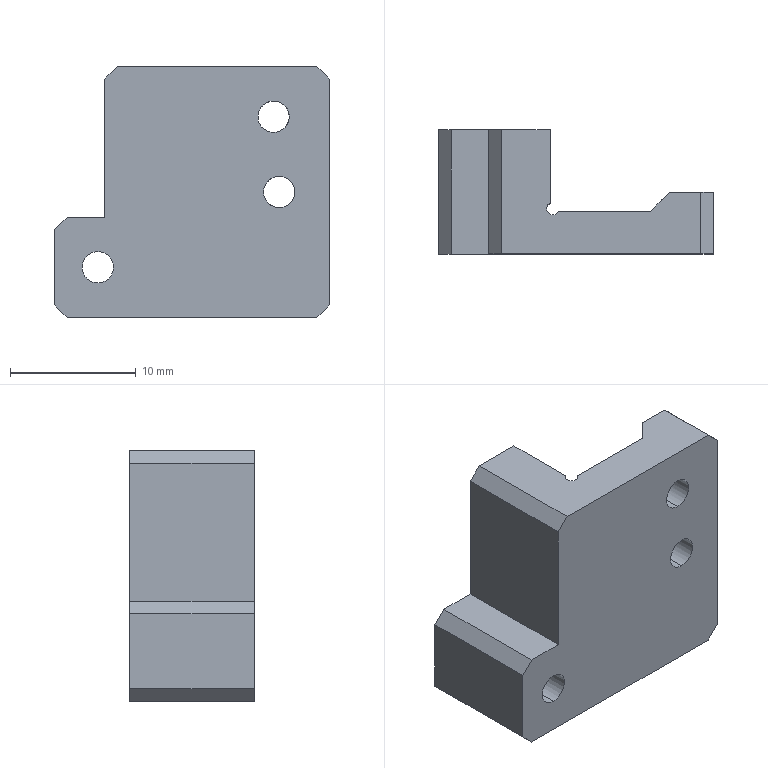Part | SolidWorks | features HoleWzd 3, ICE 2, MoveFace 2, Chamfer 1, Extrusion 1 | 1 solid | 31 faces | box 21.9 x 9.9 x 20 mm | volume 2171 mm3 | plane 19 | cylinder 10 | cone 2 | commonest cylinder face diameters 2.5 x6 1 x2 1.5 x2
STEP:
#1=CARTESIAN_POINT('',(11.9,1.75,5.75));
#2=VERTEX_POINT('',#1);
#3=CARTESIAN_POINT('',(11.9,1.75,4.25));
#4=VERTEX_POINT('',#3);
#5=CARTESIAN_POINT('',(11.9,1.75,5.));
#6=DIRECTION('',(1.,0.,0.));
#7=DIRECTION('',(0.,0.,-1.));
#8=AXIS2_PLACEMENT_3D('',#5,#6,#7);
#9=CIRCLE('',#8,0.75);
#10=EDGE_CURVE('',#2,#4,#9,.T.);
#11=ORIENTED_EDGE('',*,*,#10,.F.);
#12=CARTESIAN_POINT('',(17.9,1.75,5.75));
#13=VERTEX_POINT('',#12);
#14=CARTESIAN_POINT('',(17.9,1.75,5.75));
#15=DIRECTION('',(1.,0.,0.));
#16=VECTOR('',#15,1000.);
#17=LINE('',#14,#16);
#18=EDGE_CURVE('',#2,#13,#17,.T.);
#19=ORIENTED_EDGE('',*,*,#18,.T.);
#20=CARTESIAN_POINT('',(17.9,1.75,4.25));
#21=VERTEX_POINT('',#20);
#22=CARTESIAN_POINT('',(17.9,1.75,5.));
#23=DIRECTION('',(1.,0.,0.));
#24=DIRECTION('',(0.,0.,-1.));
#25=AXIS2_PLACEMENT_3D('',#22,#23,#24);
#26=CIRCLE('',#25,0.75);
#27=EDGE_CURVE('',#13,#21,#26,.T.);
#28=ORIENTED_EDGE('',*,*,#27,.T.);
#29=CARTESIAN_POINT('',(17.9,1.75,4.25));
#30=DIRECTION('',(1.,0.,0.));
#31=VECTOR('',#30,1000.);
#32=LINE('',#29,#31);
#33=EDGE_CURVE('',#4,#21,#32,.T.);
#34=ORIENTED_EDGE('',*,*,#33,.F.);
#35=EDGE_LOOP('',(#11,#19,#28,#34));
#36=FACE_OUTER_BOUND('',#35,.T.);
#37=CARTESIAN_POINT('',(17.9,1.75,5.));
#38=DIRECTION('',(1.,0.,0.));
#39=DIRECTION('',(0.,0.,-1.));
#40=AXIS2_PLACEMENT_3D('',#37,#38,#39);
#41=CYLINDRICAL_SURFACE('',#40,0.75);
#42=ADVANCED_FACE('',(#36),#41,.F.);
#43=CARTESIAN_POINT('',(11.449,1.75,5.));
#44=VERTEX_POINT('',#43);
#45=CARTESIAN_POINT('',(11.9,1.75,4.25));
#46=DIRECTION('',(0.515,0.,-0.8572));
#47=VECTOR('',#46,1000.);
#48=LINE('',#45,#47);
#49=EDGE_CURVE('',#44,#4,#48,.T.);
#50=ORIENTED_EDGE('',*,*,#49,.F.);
#51=CARTESIAN_POINT('',(11.9,1.75,5.75));
#52=DIRECTION('',(0.515,0.,0.8572));
#53=VECTOR('',#52,1000.);
#54=LINE('',#51,#53);
#55=EDGE_CURVE('',#44,#2,#54,.T.);
#56=ORIENTED_EDGE('',*,*,#55,.T.);
#57=ORIENTED_EDGE('',*,*,#10,.T.);
#58=EDGE_LOOP('',(#50,#56,#57));
#59=FACE_OUTER_BOUND('',#58,.T.);
#60=CARTESIAN_POINT('',(11.9,1.75,5.));
#61=DIRECTION('',(1.,0.,0.));
#62=DIRECTION('',(0.,0.,-1.));
#63=AXIS2_PLACEMENT_3D('',#60,#61,#62);
#64=CONICAL_SURFACE('',#63,0.75,1.03);
#65=ADVANCED_FACE('',(#59),#64,.F.);
#66=CARTESIAN_POINT('',(12.9,3.4,17.122));
#67=VERTEX_POINT('',#66);
#68=CARTESIAN_POINT('',(13.45,3.95,17.25));
#69=VERTEX_POINT('',#68);
#70=CARTESIAN_POINT('',(12.9,3.4,17.122));
#71=CARTESIAN_POINT('',(13.072,3.572,17.207));
#72=CARTESIAN_POINT('',(13.259,3.759,17.25));
#73=CARTESIAN_POINT('',(13.45,3.95,17.25));
#74=(BOUNDED_CURVE()B_SPLINE_CURVE(3,(#70,#71,#72,#73),.UNSPECIFIED.,.F.,.F.)B_SPLINE_CURVE_WITH_KNOTS((4,4),(1.115,1.571),.UNSPECIFIED.)CURVE()GEOMETRIC_REPRESENTATION_ITEM()RATIONAL_B_SPLINE_CURVE((1.,0.9828,0.9828,1.))REPRESENTATION_ITEM(''));
#75=EDGE_CURVE('',#67,#69,#74,.T.);
#76=ORIENTED_EDGE('',*,*,#75,.T.);
#77=CARTESIAN_POINT('',(13.45,0.,17.25));
#78=VERTEX_POINT('',#77);
#79=CARTESIAN_POINT('',(13.45,0.,17.25));
#80=DIRECTION('',(0.,-1.,0.));
#81=VECTOR('',#80,1000.);
#82=LINE('',#79,#81);
#83=EDGE_CURVE('',#69,#78,#82,.T.);
#84=ORIENTED_EDGE('',*,*,#83,.T.);
#85=CARTESIAN_POINT('',(13.45,0.,14.75));
#86=VERTEX_POINT('',#85);
#87=CARTESIAN_POINT('',(13.45,0.,16.));
#88=DIRECTION('',(0.,-1.,0.));
#89=DIRECTION('',(0.,0.,-1.));
#90=AXIS2_PLACEMENT_3D('',#87,#88,#89);
#91=CIRCLE('',#90,1.25);
#92=EDGE_CURVE('',#78,#86,#91,.T.);
#93=ORIENTED_EDGE('',*,*,#92,.T.);
#94=CARTESIAN_POINT('',(13.45,3.95,14.75));
#95=VERTEX_POINT('',#94);
#96=CARTESIAN_POINT('',(13.45,0.,14.75));
#97=DIRECTION('',(0.,-1.,0.));
#98=VECTOR('',#97,1000.);
#99=LINE('',#96,#98);
#100=EDGE_CURVE('',#95,#86,#99,.T.);
#101=ORIENTED_EDGE('',*,*,#100,.F.);
#102=CARTESIAN_POINT('',(12.9,3.4,14.878));
#103=VERTEX_POINT('',#102);
#104=CARTESIAN_POINT('',(13.45,3.95,14.75));
#105=CARTESIAN_POINT('',(13.259,3.759,14.75));
#106=CARTESIAN_POINT('',(13.072,3.572,14.793));
#107=CARTESIAN_POINT('',(12.9,3.4,14.878));
#108=(BOUNDED_CURVE()B_SPLINE_CURVE(3,(#104,#105,#106,#107),.UNSPECIFIED.,.F.,.F.)B_SPLINE_CURVE_WITH_KNOTS((4,4),(4.712,5.168),.UNSPECIFIED.)CURVE()GEOMETRIC_REPRESENTATION_ITEM()RATIONAL_B_SPLINE_CURVE((1.,0.9828,0.9828,1.))REPRESENTATION_ITEM(''));
#109=EDGE_CURVE('',#95,#103,#108,.T.);
#110=ORIENTED_EDGE('',*,*,#109,.T.);
#111=CARTESIAN_POINT('',(13.45,3.4,16.));
#112=DIRECTION('',(0.,-1.,0.));
#113=DIRECTION('',(1.,0.,0.));
#114=AXIS2_PLACEMENT_3D('',#111,#112,#113);
#115=CIRCLE('',#114,1.25);
#116=EDGE_CURVE('',#67,#103,#115,.T.);
#117=ORIENTED_EDGE('',*,*,#116,.F.);
#118=EDGE_LOOP('',(#76,#84,#93,#101,#110,#117));
#119=FACE_OUTER_BOUND('',#118,.T.);
#120=CARTESIAN_POINT('',(13.45,0.,16.));
#121=DIRECTION('',(0.,-1.,0.));
#122=DIRECTION('',(0.,0.,-1.));
#123=AXIS2_PLACEMENT_3D('',#120,#121,#122);
#124=CYLINDRICAL_SURFACE('',#123,1.25);
#125=ADVANCED_FACE('',(#119),#124,.F.);
#126=CARTESIAN_POINT('',(-0.55,9.9,5.25));
#127=VERTEX_POINT('',#126);
#128=CARTESIAN_POINT('',(-0.55,9.9,2.75));
#129=VERTEX_POINT('',#128);
#130=CARTESIAN_POINT('',(-0.55,9.9,4.));
#131=DIRECTION('',(0.,-1.,0.));
#132=DIRECTION('',(0.,0.,-1.));
#133=AXIS2_PLACEMENT_3D('',#130,#131,#132);
#134=CIRCLE('',#133,1.25);
#135=EDGE_CURVE('',#127,#129,#134,.T.);
#136=ORIENTED_EDGE('',*,*,#135,.F.);
#137=CARTESIAN_POINT('',(-0.55,0.,5.25));
#138=VERTEX_POINT('',#137);
#139=CARTESIAN_POINT('',(-0.55,0.,5.25));
#140=DIRECTION('',(0.,-1.,0.));
#141=VECTOR('',#140,1000.);
#142=LINE('',#139,#141);
#143=EDGE_CURVE('',#127,#138,#142,.T.);
#144=ORIENTED_EDGE('',*,*,#143,.T.);
#145=CARTESIAN_POINT('',(-0.55,0.,2.75));
#146=VERTEX_POINT('',#145);
#147=CARTESIAN_POINT('',(-0.55,0.,4.));
#148=DIRECTION('',(0.,-1.,0.));
#149=DIRECTION('',(0.,0.,-1.));
#150=AXIS2_PLACEMENT_3D('',#147,#148,#149);
#151=CIRCLE('',#150,1.25);
#152=EDGE_CURVE('',#138,#146,#151,.T.);
#153=ORIENTED_EDGE('',*,*,#152,.T.);
#154=CARTESIAN_POINT('',(-0.55,0.,2.75));
#155=DIRECTION('',(0.,-1.,0.));
#156=VECTOR('',#155,1000.);
#157=LINE('',#154,#156);
#158=EDGE_CURVE('',#129,#146,#157,.T.);
#159=ORIENTED_EDGE('',*,*,#158,.F.);
#160=EDGE_LOOP('',(#136,#144,#153,#159));
#161=FACE_OUTER_BOUND('',#160,.T.);
#162=CARTESIAN_POINT('',(-0.55,0.,4.));
#163=DIRECTION('',(0.,-1.,0.));
#164=DIRECTION('',(0.,0.,-1.));
#165=AXIS2_PLACEMENT_3D('',#162,#163,#164);
#166=CYLINDRICAL_SURFACE('',#165,1.25);
#167=ADVANCED_FACE('',(#161),#166,.F.);
#168=CARTESIAN_POINT('',(12.9,3.4,10.75));
#169=VERTEX_POINT('',#168);
#170=CARTESIAN_POINT('',(13.9,4.4,11.25));
#171=VERTEX_POINT('',#170);
#172=CARTESIAN_POINT('',(12.9,3.4,10.75));
#173=CARTESIAN_POINT('',(13.141,3.641,11.071));
#174=CARTESIAN_POINT('',(13.499,3.999,11.25));
#175=CARTESIAN_POINT('',(13.9,4.4,11.25));
#176=(BOUNDED_CURVE()B_SPLINE_CURVE(3,(#172,#173,#174,#175),.UNSPECIFIED.,.F.,.F.)B_SPLINE_CURVE_WITH_KNOTS((4,4),(0.6435,1.571),.UNSPECIFIED.)CURVE()GEOMETRIC_REPRESENTATION_ITEM()RATIONAL_B_SPLINE_CURVE((1.,0.9296,0.9296,1.))REPRESENTATION_ITEM(''));
#177=EDGE_CURVE('',#169,#171,#176,.T.);
#178=ORIENTED_EDGE('',*,*,#177,.T.);
#179=CARTESIAN_POINT('',(13.9,0.,11.25));
#180=VERTEX_POINT('',#179);
#181=CARTESIAN_POINT('',(13.9,0.,11.25));
#182=DIRECTION('',(0.,-1.,0.));
#183=VECTOR('',#182,1000.);
#184=LINE('',#181,#183);
#185=EDGE_CURVE('',#171,#180,#184,.T.);
#186=ORIENTED_EDGE('',*,*,#185,.T.);
#187=CARTESIAN_POINT('',(13.9,0.,8.75));
#188=VERTEX_POINT('',#187);
#189=CARTESIAN_POINT('',(13.9,0.,10.));
#190=DIRECTION('',(0.,-1.,0.));
#191=DIRECTION('',(0.,0.,-1.));
#192=AXIS2_PLACEMENT_3D('',#189,#190,#191);
#193=CIRCLE('',#192,1.25);
#194=EDGE_CURVE('',#180,#188,#193,.T.);
#195=ORIENTED_EDGE('',*,*,#194,.T.);
#196=CARTESIAN_POINT('',(13.9,4.4,8.75));
#197=VERTEX_POINT('',#196);
#198=CARTESIAN_POINT('',(13.9,0.,8.75));
#199=DIRECTION('',(0.,-1.,0.));
#200=VECTOR('',#199,1000.);
#201=LINE('',#198,#200);
#202=EDGE_CURVE('',#197,#188,#201,.T.);
#203=ORIENTED_EDGE('',*,*,#202,.F.);
#204=CARTESIAN_POINT('',(12.9,3.4,9.25));
#205=VERTEX_POINT('',#204);
#206=CARTESIAN_POINT('',(13.9,4.4,8.75));
#207=CARTESIAN_POINT('',(13.499,3.999,8.75));
#208=CARTESIAN_POINT('',(13.141,3.641,8.929));
#209=CARTESIAN_POINT('',(12.9,3.4,9.25));
#210=(BOUNDED_CURVE()B_SPLINE_CURVE(3,(#206,#207,#208,#209),.UNSPECIFIED.,.F.,.T.)B_SPLINE_CURVE_WITH_KNOTS((4,4),(4.712,5.64),.UNSPECIFIED.)CURVE()GEOMETRIC_REPRESENTATION_ITEM()RATIONAL_B_SPLINE_CURVE((1.,0.9296,0.9296,1.))REPRESENTATION_ITEM(''));
#211=EDGE_CURVE('',#197,#205,#210,.T.);
#212=ORIENTED_EDGE('',*,*,#211,.T.);
#213=CARTESIAN_POINT('',(13.9,3.4,10.));
#214=DIRECTION('',(0.,-1.,0.));
#215=DIRECTION('',(1.,0.,0.));
#216=AXIS2_PLACEMENT_3D('',#213,#214,#215);
#217=CIRCLE('',#216,1.25);
#218=EDGE_CURVE('',#169,#205,#217,.T.);
#219=ORIENTED_EDGE('',*,*,#218,.F.);
#220=EDGE_LOOP('',(#178,#186,#195,#203,#212,#219));
#221=FACE_OUTER_BOUND('',#220,.T.);
#222=CARTESIAN_POINT('',(13.9,0.,10.));
#223=DIRECTION('',(0.,-1.,0.));
#224=DIRECTION('',(0.,0.,-1.));
#225=AXIS2_PLACEMENT_3D('',#222,#223,#224);
#226=CYLINDRICAL_SURFACE('',#225,1.25);
#227=ADVANCED_FACE('',(#221),#226,.F.);
#228=CARTESIAN_POINT('',(4.6,3.6,20.));
#229=VERTEX_POINT('',#228);
#230=CARTESIAN_POINT('',(4.9,4.058,20.));
#231=VERTEX_POINT('',#230);
#232=CARTESIAN_POINT('',(5.1,3.6,20.));
#233=DIRECTION('',(0.,0.,-1.));
#234=DIRECTION('',(1.,0.,0.));
#235=AXIS2_PLACEMENT_3D('',#232,#233,#234);
#236=CIRCLE('',#235,0.5);
#237=EDGE_CURVE('',#229,#231,#236,.T.);
#238=ORIENTED_EDGE('',*,*,#237,.F.);
#239=CARTESIAN_POINT('',(4.6,3.6,0.));
#240=VERTEX_POINT('',#239);
#241=CARTESIAN_POINT('',(4.6,3.6,20.));
#242=DIRECTION('',(0.,0.,-1.));
#243=VECTOR('',#242,1000.);
#244=LINE('',#241,#243);
#245=EDGE_CURVE('',#229,#240,#244,.T.);
#246=ORIENTED_EDGE('',*,*,#245,.T.);
#247=CARTESIAN_POINT('',(4.9,4.058,0.));
#248=VERTEX_POINT('',#247);
#249=CARTESIAN_POINT('',(5.1,3.6,0.));
#250=DIRECTION('',(0.,0.,-1.));
#251=DIRECTION('',(1.,0.,0.));
#252=AXIS2_PLACEMENT_3D('',#249,#250,#251);
#253=CIRCLE('',#252,0.5);
#254=EDGE_CURVE('',#240,#248,#253,.T.);
#255=ORIENTED_EDGE('',*,*,#254,.T.);
#256=CARTESIAN_POINT('',(4.9,4.058,20.));
#257=DIRECTION('',(0.,0.,-1.));
#258=VECTOR('',#257,1000.);
#259=LINE('',#256,#258);
#260=EDGE_CURVE('',#231,#248,#259,.T.);
#261=ORIENTED_EDGE('',*,*,#260,.F.);
#262=EDGE_LOOP('',(#238,#246,#255,#261));
#263=FACE_OUTER_BOUND('',#262,.T.);
#264=CARTESIAN_POINT('',(5.1,3.6,20.));
#265=DIRECTION('',(0.,0.,-1.));
#266=DIRECTION('',(-1.,0.,0.));
#267=AXIS2_PLACEMENT_3D('',#264,#265,#266);
#268=CYLINDRICAL_SURFACE('',#267,0.5);
#269=ADVANCED_FACE('',(#263),#268,.F.);
#270=ORIENTED_EDGE('',*,*,#75,.F.);
#271=CARTESIAN_POINT('',(12.9,3.4,20.));
#272=VERTEX_POINT('',#271);
#273=CARTESIAN_POINT('',(12.9,3.4,25.22));
#274=DIRECTION('',(0.,0.,-1.));
#275=VECTOR('',#274,1000.);
#276=LINE('',#273,#275);
#277=EDGE_CURVE('',#272,#67,#276,.T.);
#278=ORIENTED_EDGE('',*,*,#277,.F.);
#279=CARTESIAN_POINT('',(14.4,4.9,20.));
#280=VERTEX_POINT('',#279);
#281=CARTESIAN_POINT('',(14.4,4.9,20.));
#282=DIRECTION('',(0.7071,0.7071,0.));
#283=VECTOR('',#282,1000.);
#284=LINE('',#281,#283);
#285=EDGE_CURVE('',#272,#280,#284,.T.);
#286=ORIENTED_EDGE('',*,*,#285,.T.);
#287=CARTESIAN_POINT('',(14.4,4.9,16.812));
#288=VERTEX_POINT('',#287);
#289=CARTESIAN_POINT('',(14.4,4.9,25.22));
#290=DIRECTION('',(0.,0.,-1.));
#291=VECTOR('',#290,1000.);
#292=LINE('',#289,#291);
#293=EDGE_CURVE('',#280,#288,#292,.T.);
#294=ORIENTED_EDGE('',*,*,#293,.T.);
#295=CARTESIAN_POINT('',(13.45,3.95,17.25));
#296=CARTESIAN_POINT('',(13.821,4.321,17.25));
#297=CARTESIAN_POINT('',(14.159,4.659,17.095));
#298=CARTESIAN_POINT('',(14.4,4.9,16.812));
#299=(BOUNDED_CURVE()B_SPLINE_CURVE(3,(#295,#296,#297,#298),.UNSPECIFIED.,.F.,.T.)B_SPLINE_CURVE_WITH_KNOTS((4,4),(1.571,2.434),.UNSPECIFIED.)CURVE()GEOMETRIC_REPRESENTATION_ITEM()RATIONAL_B_SPLINE_CURVE((1.,0.9388,0.9388,1.))REPRESENTATION_ITEM(''));
#300=EDGE_CURVE('',#69,#288,#299,.T.);
#301=ORIENTED_EDGE('',*,*,#300,.F.);
#302=EDGE_LOOP('',(#270,#278,#286,#294,#301));
#303=FACE_OUTER_BOUND('',#302,.T.);
#304=CARTESIAN_POINT('',(14.4,4.9,25.22));
#305=DIRECTION('',(-0.7071,0.7071,0.));
#306=DIRECTION('',(-0.7071,-0.7071,0.));
#307=AXIS2_PLACEMENT_3D('',#304,#305,#306);
#308=PLANE('',#307);
#309=ADVANCED_FACE('',(#303),#308,.T.);
#310=CARTESIAN_POINT('',(14.4,4.9,15.188));
#311=VERTEX_POINT('',#310);
#312=CARTESIAN_POINT('',(14.4,4.9,15.188));
#313=CARTESIAN_POINT('',(14.159,4.659,14.905));
#314=CARTESIAN_POINT('',(13.821,4.321,14.75));
#315=CARTESIAN_POINT('',(13.45,3.95,14.75));
#316=(BOUNDED_CURVE()B_SPLINE_CURVE(3,(#312,#313,#314,#315),.UNSPECIFIED.,.F.,.F.)B_SPLINE_CURVE_WITH_KNOTS((4,4),(3.849,4.712),.UNSPECIFIED.)CURVE()GEOMETRIC_REPRESENTATION_ITEM()RATIONAL_B_SPLINE_CURVE((1.,0.9388,0.9388,1.))REPRESENTATION_ITEM(''));
#317=EDGE_CURVE('',#311,#95,#316,.T.);
#318=ORIENTED_EDGE('',*,*,#317,.F.);
#319=CARTESIAN_POINT('',(14.4,4.9,11.146));
#320=VERTEX_POINT('',#319);
#321=CARTESIAN_POINT('',(14.4,4.9,25.22));
#322=DIRECTION('',(0.,0.,-1.));
#323=VECTOR('',#322,1000.);
#324=LINE('',#321,#323);
#325=EDGE_CURVE('',#311,#320,#324,.T.);
#326=ORIENTED_EDGE('',*,*,#325,.T.);
#327=CARTESIAN_POINT('',(13.9,4.4,11.25));
#328=CARTESIAN_POINT('',(14.073,4.573,11.25));
#329=CARTESIAN_POINT('',(14.242,4.742,11.215));
#330=CARTESIAN_POINT('',(14.4,4.9,11.146));
#331=(BOUNDED_CURVE()B_SPLINE_CURVE(3,(#327,#328,#329,#330),.UNSPECIFIED.,.F.,.T.)B_SPLINE_CURVE_WITH_KNOTS((4,4),(1.571,1.982),.UNSPECIFIED.)CURVE()GEOMETRIC_REPRESENTATION_ITEM()RATIONAL_B_SPLINE_CURVE((1.,0.9859,0.9859,1.))REPRESENTATION_ITEM(''));
#332=EDGE_CURVE('',#171,#320,#331,.T.);
#333=ORIENTED_EDGE('',*,*,#332,.F.);
#334=ORIENTED_EDGE('',*,*,#177,.F.);
#335=CARTESIAN_POINT('',(12.9,3.4,25.22));
#336=DIRECTION('',(0.,0.,-1.));
#337=VECTOR('',#336,1000.);
#338=LINE('',#335,#337);
#339=EDGE_CURVE('',#103,#169,#338,.T.);
#340=ORIENTED_EDGE('',*,*,#339,.F.);
#341=ORIENTED_EDGE('',*,*,#109,.F.);
#342=EDGE_LOOP('',(#318,#326,#333,#334,#340,#341));
#343=FACE_OUTER_BOUND('',#342,.T.);
#344=CARTESIAN_POINT('',(14.4,4.9,25.22));
#345=DIRECTION('',(-0.7071,0.7071,0.));
#346=DIRECTION('',(-0.7071,-0.7071,0.));
#347=AXIS2_PLACEMENT_3D('',#344,#345,#346);
#348=PLANE('',#347);
#349=ADVANCED_FACE('',(#343),#348,.T.);
#350=CARTESIAN_POINT('',(13.45,0.,16.));
#351=DIRECTION('',(0.,-1.,0.));
#352=DIRECTION('',(0.,0.,-1.));
#353=AXIS2_PLACEMENT_3D('',#350,#351,#352);
#354=CIRCLE('',#353,1.25);
#355=EDGE_CURVE('',#86,#78,#354,.T.);
#356=ORIENTED_EDGE('',*,*,#355,.F.);
#357=ORIENTED_EDGE('',*,*,#92,.F.);
#358=EDGE_LOOP('',(#356,#357));
#359=FACE_BOUND('',#358,.T.);
#360=CARTESIAN_POINT('',(-0.55,0.,4.));
#361=DIRECTION('',(0.,-1.,0.));
#362=DIRECTION('',(0.,0.,-1.));
#363=AXIS2_PLACEMENT_3D('',#360,#361,#362);
#364=CIRCLE('',#363,1.25);
#365=EDGE_CURVE('',#146,#138,#364,.T.);
#366=ORIENTED_EDGE('',*,*,#365,.F.);
#367=ORIENTED_EDGE('',*,*,#152,.F.);
#368=EDGE_LOOP('',(#366,#367));
#369=FACE_BOUND('',#368,.T.);
#370=CARTESIAN_POINT('',(13.9,0.,10.));
#371=DIRECTION('',(0.,-1.,0.));
#372=DIRECTION('',(0.,0.,-1.));
#373=AXIS2_PLACEMENT_3D('',#370,#371,#372);
#374=CIRCLE('',#373,1.25);
#375=EDGE_CURVE('',#188,#180,#374,.T.);
#376=ORIENTED_EDGE('',*,*,#375,.F.);
#377=ORIENTED_EDGE('',*,*,#194,.F.);
#378=EDGE_LOOP('',(#376,#377));
#379=FACE_BOUND('',#378,.T.);
#380=CARTESIAN_POINT('',(-3.,0.,0.));
#381=VERTEX_POINT('',#380);
#382=CARTESIAN_POINT('',(16.9,0.,0.));
#383=VERTEX_POINT('',#382);
#384=CARTESIAN_POINT('',(8.,0.,0.));
#385=DIRECTION('',(1.,0.,0.));
#386=VECTOR('',#385,1000.);
#387=LINE('',#384,#386);
#388=EDGE_CURVE('',#381,#383,#387,.T.);
#389=ORIENTED_EDGE('',*,*,#388,.T.);
#390=CARTESIAN_POINT('',(17.9,0.,1.));
#391=VERTEX_POINT('',#390);
#392=CARTESIAN_POINT('',(17.9,0.,1.));
#393=DIRECTION('',(0.7071,0.,0.7071));
#394=VECTOR('',#393,1000.);
#395=LINE('',#392,#394);
#396=EDGE_CURVE('',#383,#391,#395,.T.);
#397=ORIENTED_EDGE('',*,*,#396,.T.);
#398=CARTESIAN_POINT('',(17.9,0.,19.));
#399=VERTEX_POINT('',#398);
#400=CARTESIAN_POINT('',(17.9,0.,20.));
#401=DIRECTION('',(0.,0.,-1.));
#402=VECTOR('',#401,1000.);
#403=LINE('',#400,#402);
#404=EDGE_CURVE('',#399,#391,#403,.T.);
#405=ORIENTED_EDGE('',*,*,#404,.F.);
#406=CARTESIAN_POINT('',(16.9,0.,20.));
#407=VERTEX_POINT('',#406);
#408=CARTESIAN_POINT('',(16.9,0.,20.));
#409=DIRECTION('',(-0.7071,0.,0.7071));
#410=VECTOR('',#409,1000.);
#411=LINE('',#408,#410);
#412=EDGE_CURVE('',#399,#407,#411,.T.);
#413=ORIENTED_EDGE('',*,*,#412,.T.);
#414=CARTESIAN_POINT('',(1.,0.,20.));
#415=VERTEX_POINT('',#414);
#416=CARTESIAN_POINT('',(8.,0.,20.));
#417=DIRECTION('',(1.,0.,0.));
#418=VECTOR('',#417,1000.);
#419=LINE('',#416,#418);
#420=EDGE_CURVE('',#415,#407,#419,.T.);
#421=ORIENTED_EDGE('',*,*,#420,.F.);
#422=CARTESIAN_POINT('',(0.,0.,19.));
#423=VERTEX_POINT('',#422);
#424=CARTESIAN_POINT('',(1.,0.,20.));
#425=DIRECTION('',(-0.7071,0.,-0.7071));
#426=VECTOR('',#425,1000.);
#427=LINE('',#424,#426);
#428=EDGE_CURVE('',#415,#423,#427,.T.);
#429=ORIENTED_EDGE('',*,*,#428,.T.);
#430=CARTESIAN_POINT('',(0.,0.,8.));
#431=VERTEX_POINT('',#430);
#432=CARTESIAN_POINT('',(0.,0.,20.));
#433=DIRECTION('',(0.,0.,-1.));
#434=VECTOR('',#433,1000.);
#435=LINE('',#432,#434);
#436=EDGE_CURVE('',#423,#431,#435,.T.);
#437=ORIENTED_EDGE('',*,*,#436,.T.);
#438=CARTESIAN_POINT('',(-3.,0.,8.));
#439=VERTEX_POINT('',#438);
#440=CARTESIAN_POINT('',(-4.,0.,8.));
#441=DIRECTION('',(-1.,0.,0.));
#442=VECTOR('',#441,1000.);
#443=LINE('',#440,#442);
#444=EDGE_CURVE('',#431,#439,#443,.T.);
#445=ORIENTED_EDGE('',*,*,#444,.T.);
#446=CARTESIAN_POINT('',(-4.,0.,7.));
#447=VERTEX_POINT('',#446);
#448=CARTESIAN_POINT('',(-3.,0.,8.));
#449=DIRECTION('',(-0.7071,0.,-0.7071));
#450=VECTOR('',#449,1000.);
#451=LINE('',#448,#450);
#452=EDGE_CURVE('',#439,#447,#451,.T.);
#453=ORIENTED_EDGE('',*,*,#452,.T.);
#454=CARTESIAN_POINT('',(-4.,0.,1.));
#455=VERTEX_POINT('',#454);
#456=CARTESIAN_POINT('',(-4.,0.,8.));
#457=DIRECTION('',(0.,0.,-1.));
#458=VECTOR('',#457,1000.);
#459=LINE('',#456,#458);
#460=EDGE_CURVE('',#447,#455,#459,.T.);
#461=ORIENTED_EDGE('',*,*,#460,.T.);
#462=CARTESIAN_POINT('',(-4.,0.,1.));
#463=DIRECTION('',(0.7071,0.,-0.7071));
#464=VECTOR('',#463,1000.);
#465=LINE('',#462,#464);
#466=EDGE_CURVE('',#455,#381,#465,.T.);
#467=ORIENTED_EDGE('',*,*,#466,.T.);
#468=EDGE_LOOP('',(#389,#397,#405,#413,#421,#429,#437,#445,#453,#461,#467));
#469=FACE_OUTER_BOUND('',#468,.T.);
#470=CARTESIAN_POINT('',(8.,0.,20.));
#471=DIRECTION('',(0.,1.,0.));
#472=DIRECTION('',(-1.,0.,0.));
#473=AXIS2_PLACEMENT_3D('',#470,#471,#472);
#474=PLANE('',#473);
#475=ADVANCED_FACE('',(#359,#369,#379,#469),#474,.F.);
#476=CARTESIAN_POINT('',(17.9,1.75,5.));
#477=DIRECTION('',(1.,0.,0.));
#478=DIRECTION('',(0.,0.,-1.));
#479=AXIS2_PLACEMENT_3D('',#476,#477,#478);
#480=CIRCLE('',#479,0.75);
#481=EDGE_CURVE('',#21,#13,#480,.T.);
#482=ORIENTED_EDGE('',*,*,#481,.F.);
#483=ORIENTED_EDGE('',*,*,#27,.F.);
#484=EDGE_LOOP('',(#482,#483));
#485=FACE_BOUND('',#484,.T.);
#486=ORIENTED_EDGE('',*,*,#404,.T.);
#487=CARTESIAN_POINT('',(17.9,4.9,1.));
#488=VERTEX_POINT('',#487);
#489=CARTESIAN_POINT('',(17.9,3.4,1.));
#490=DIRECTION('',(0.,1.,0.));
#491=VECTOR('',#490,1000.);
#492=LINE('',#489,#491);
#493=EDGE_CURVE('',#391,#488,#492,.T.);
#494=ORIENTED_EDGE('',*,*,#493,.T.);
#495=CARTESIAN_POINT('',(17.9,4.9,19.));
#496=VERTEX_POINT('',#495);
#497=CARTESIAN_POINT('',(17.9,4.9,25.22));
#498=DIRECTION('',(0.,0.,-1.));
#499=VECTOR('',#498,1000.);
#500=LINE('',#497,#499);
#501=EDGE_CURVE('',#496,#488,#500,.T.);
#502=ORIENTED_EDGE('',*,*,#501,.F.);
#503=CARTESIAN_POINT('',(17.9,0.,19.));
#504=DIRECTION('',(0.,-1.,0.));
#505=VECTOR('',#504,1000.);
#506=LINE('',#503,#505);
#507=EDGE_CURVE('',#496,#399,#506,.T.);
#508=ORIENTED_EDGE('',*,*,#507,.T.);
#509=EDGE_LOOP('',(#486,#494,#502,#508));
#510=FACE_OUTER_BOUND('',#509,.T.);
#511=CARTESIAN_POINT('',(17.9,3.4,20.));
#512=DIRECTION('',(-1.,0.,0.));
#513=DIRECTION('',(0.,0.,1.));
#514=AXIS2_PLACEMENT_3D('',#511,#512,#513);
#515=PLANE('',#514);
#516=ADVANCED_FACE('',(#485,#510),#515,.F.);
#517=ORIENTED_EDGE('',*,*,#277,.T.);
#518=ORIENTED_EDGE('',*,*,#116,.T.);
#519=ORIENTED_EDGE('',*,*,#339,.T.);
#520=ORIENTED_EDGE('',*,*,#218,.T.);
#521=CARTESIAN_POINT('',(12.9,3.4,0.));
#522=VERTEX_POINT('',#521);
#523=CARTESIAN_POINT('',(12.9,3.4,25.22));
#524=DIRECTION('',(0.,0.,-1.));
#525=VECTOR('',#524,1000.);
#526=LINE('',#523,#525);
#527=EDGE_CURVE('',#205,#522,#526,.T.);
#528=ORIENTED_EDGE('',*,*,#527,.T.);
#529=CARTESIAN_POINT('',(5.558,3.4,0.));
#530=VERTEX_POINT('',#529);
#531=CARTESIAN_POINT('',(5.558,3.4,0.));
#532=DIRECTION('',(-1.,0.,0.));
#533=VECTOR('',#532,1000.);
#534=LINE('',#531,#533);
#535=EDGE_CURVE('',#522,#530,#534,.T.);
#536=ORIENTED_EDGE('',*,*,#535,.T.);
#537=CARTESIAN_POINT('',(5.558,3.4,20.));
#538=VERTEX_POINT('',#537);
#539=CARTESIAN_POINT('',(5.558,3.4,20.));
#540=DIRECTION('',(0.,0.,-1.));
#541=VECTOR('',#540,1000.);
#542=LINE('',#539,#541);
#543=EDGE_CURVE('',#538,#530,#542,.T.);
#544=ORIENTED_EDGE('',*,*,#543,.F.);
#545=CARTESIAN_POINT('',(5.558,3.4,20.));
#546=DIRECTION('',(-1.,0.,0.));
#547=VECTOR('',#546,1000.);
#548=LINE('',#545,#547);
#549=EDGE_CURVE('',#272,#538,#548,.T.);
#550=ORIENTED_EDGE('',*,*,#549,.F.);
#551=EDGE_LOOP('',(#517,#518,#519,#520,#528,#536,#544,#550));
#552=FACE_OUTER_BOUND('',#551,.T.);
#553=CARTESIAN_POINT('',(5.558,3.4,20.));
#554=DIRECTION('',(0.,-1.,0.));
#555=DIRECTION('',(1.,0.,0.));
#556=AXIS2_PLACEMENT_3D('',#553,#554,#555);
#557=PLANE('',#556);
#558=ADVANCED_FACE('',(#552),#557,.F.);
#559=ORIENTED_EDGE('',*,*,#245,.F.);
#560=CARTESIAN_POINT('',(5.1,3.6,20.));
#561=DIRECTION('',(0.,0.,-1.));
#562=DIRECTION('',(1.,0.,0.));
#563=AXIS2_PLACEMENT_3D('',#560,#561,#562);
#564=CIRCLE('',#563,0.5);
#565=EDGE_CURVE('',#538,#229,#564,.T.);
#566=ORIENTED_EDGE('',*,*,#565,.F.);
#567=ORIENTED_EDGE('',*,*,#543,.T.);
#568=CARTESIAN_POINT('',(5.1,3.6,0.));
#569=DIRECTION('',(0.,0.,-1.));
#570=DIRECTION('',(1.,0.,0.));
#571=AXIS2_PLACEMENT_3D('',#568,#569,#570);
#572=CIRCLE('',#571,0.5);
#573=EDGE_CURVE('',#530,#240,#572,.T.);
#574=ORIENTED_EDGE('',*,*,#573,.T.);
#575=EDGE_LOOP('',(#559,#566,#567,#574));
#576=FACE_OUTER_BOUND('',#575,.T.);
#577=CARTESIAN_POINT('',(5.1,3.6,20.));
#578=DIRECTION('',(0.,0.,-1.));
#579=DIRECTION('',(-1.,0.,0.));
#580=AXIS2_PLACEMENT_3D('',#577,#578,#579);
#581=CYLINDRICAL_SURFACE('',#580,0.5);
#582=ADVANCED_FACE('',(#576),#581,.F.);
#583=CARTESIAN_POINT('',(4.9,9.9,0.));
#584=VERTEX_POINT('',#583);
#585=CARTESIAN_POINT('',(4.9,6.5,0.));
#586=DIRECTION('',(0.,1.,0.));
#587=VECTOR('',#586,1000.);
#588=LINE('',#585,#587);
#589=EDGE_CURVE('',#248,#584,#588,.T.);
#590=ORIENTED_EDGE('',*,*,#589,.T.);
#591=CARTESIAN_POINT('',(4.9,9.9,20.));
#592=VERTEX_POINT('',#591);
#593=CARTESIAN_POINT('',(4.9,9.9,20.));
#594=DIRECTION('',(0.,0.,-1.));
#595=VECTOR('',#594,1000.);
#596=LINE('',#593,#595);
#597=EDGE_CURVE('',#592,#584,#596,.T.);
#598=ORIENTED_EDGE('',*,*,#597,.F.);
#599=CARTESIAN_POINT('',(4.9,6.5,20.));
#600=DIRECTION('',(0.,1.,0.));
#601=VECTOR('',#600,1000.);
#602=LINE('',#599,#601);
#603=EDGE_CURVE('',#231,#592,#602,.T.);
#604=ORIENTED_EDGE('',*,*,#603,.F.);
#605=ORIENTED_EDGE('',*,*,#260,.T.);
#606=EDGE_LOOP('',(#590,#598,#604,#605));
#607=FACE_OUTER_BOUND('',#606,.T.);
#608=CARTESIAN_POINT('',(4.9,6.5,20.));
#609=DIRECTION('',(-1.,0.,0.));
#610=DIRECTION('',(0.,-1.,0.));
#611=AXIS2_PLACEMENT_3D('',#608,#609,#610);
#612=PLANE('',#611);
#613=ADVANCED_FACE('',(#607),#612,.F.);
#614=CARTESIAN_POINT('',(-0.55,9.9,4.));
#615=DIRECTION('',(0.,-1.,0.));
#616=DIRECTION('',(0.,0.,-1.));
#617=AXIS2_PLACEMENT_3D('',#614,#615,#616);
#618=CIRCLE('',#617,1.25);
#619=EDGE_CURVE('',#129,#127,#618,.T.);
#620=ORIENTED_EDGE('',*,*,#619,.T.);
#621=ORIENTED_EDGE('',*,*,#135,.T.);
#622=EDGE_LOOP('',(#620,#621));
#623=FACE_BOUND('',#622,.T.);
#624=CARTESIAN_POINT('',(0.,9.9,19.));
#625=VERTEX_POINT('',#624);
#626=CARTESIAN_POINT('',(0.,9.9,8.));
#627=VERTEX_POINT('',#626);
#628=CARTESIAN_POINT('',(0.,9.9,20.));
#629=DIRECTION('',(0.,0.,-1.));
#630=VECTOR('',#629,1000.);
#631=LINE('',#628,#630);
#632=EDGE_CURVE('',#625,#627,#631,.T.);
#633=ORIENTED_EDGE('',*,*,#632,.F.);
#634=CARTESIAN_POINT('',(1.,9.9,20.));
#635=VERTEX_POINT('',#634);
#636=CARTESIAN_POINT('',(1.,9.9,20.));
#637=DIRECTION('',(0.7071,0.,0.7071));
#638=VECTOR('',#637,1000.);
#639=LINE('',#636,#638);
#640=EDGE_CURVE('',#625,#635,#639,.T.);
#641=ORIENTED_EDGE('',*,*,#640,.T.);
#642=CARTESIAN_POINT('',(0.,9.9,20.));
#643=DIRECTION('',(-1.,0.,0.));
#644=VECTOR('',#643,1000.);
#645=LINE('',#642,#644);
#646=EDGE_CURVE('',#592,#635,#645,.T.);
#647=ORIENTED_EDGE('',*,*,#646,.F.);
#648=ORIENTED_EDGE('',*,*,#597,.T.);
#649=CARTESIAN_POINT('',(-3.,9.9,0.));
#650=VERTEX_POINT('',#649);
#651=CARTESIAN_POINT('',(0.,9.9,0.));
#652=DIRECTION('',(-1.,0.,0.));
#653=VECTOR('',#652,1000.);
#654=LINE('',#651,#653);
#655=EDGE_CURVE('',#584,#650,#654,.T.);
#656=ORIENTED_EDGE('',*,*,#655,.T.);
#657=CARTESIAN_POINT('',(-4.,9.9,1.));
#658=VERTEX_POINT('',#657);
#659=CARTESIAN_POINT('',(-4.,9.9,1.));
#660=DIRECTION('',(-0.7071,0.,0.7071));
#661=VECTOR('',#660,1000.);
#662=LINE('',#659,#661);
#663=EDGE_CURVE('',#650,#658,#662,.T.);
#664=ORIENTED_EDGE('',*,*,#663,.T.);
#665=CARTESIAN_POINT('',(-4.,9.9,7.));
#666=VERTEX_POINT('',#665);
#667=CARTESIAN_POINT('',(-4.,9.9,8.));
#668=DIRECTION('',(0.,0.,1.));
#669=VECTOR('',#668,1000.);
#670=LINE('',#667,#669);
#671=EDGE_CURVE('',#658,#666,#670,.T.);
#672=ORIENTED_EDGE('',*,*,#671,.T.);
#673=CARTESIAN_POINT('',(-3.,9.9,8.));
#674=VERTEX_POINT('',#673);
#675=CARTESIAN_POINT('',(-3.,9.9,8.));
#676=DIRECTION('',(0.7071,0.,0.7071));
#677=VECTOR('',#676,1000.);
#678=LINE('',#675,#677);
#679=EDGE_CURVE('',#666,#674,#678,.T.);
#680=ORIENTED_EDGE('',*,*,#679,.T.);
#681=CARTESIAN_POINT('',(-4.,9.9,8.));
#682=DIRECTION('',(1.,0.,0.));
#683=VECTOR('',#682,1000.);
#684=LINE('',#681,#683);
#685=EDGE_CURVE('',#674,#627,#684,.T.);
#686=ORIENTED_EDGE('',*,*,#685,.T.);
#687=EDGE_LOOP('',(#633,#641,#647,#648,#656,#664,#672,#680,#686));
#688=FACE_OUTER_BOUND('',#687,.T.);
#689=CARTESIAN_POINT('',(0.,9.9,20.));
#690=DIRECTION('',(0.,-1.,0.));
#691=DIRECTION('',(0.,0.,-1.));
#692=AXIS2_PLACEMENT_3D('',#689,#690,#691);
#693=PLANE('',#692);
#694=ADVANCED_FACE('',(#623,#688),#693,.F.);
#695=ORIENTED_EDGE('',*,*,#436,.F.);
#696=CARTESIAN_POINT('',(0.,9.9,19.));
#697=DIRECTION('',(0.,1.,0.));
#698=VECTOR('',#697,1000.);
#699=LINE('',#696,#698);
#700=EDGE_CURVE('',#423,#625,#699,.T.);
#701=ORIENTED_EDGE('',*,*,#700,.T.);
#702=ORIENTED_EDGE('',*,*,#632,.T.);
#703=CARTESIAN_POINT('',(0.,18.844,8.));
#704=DIRECTION('',(0.,-1.,0.));
#705=VECTOR('',#704,1000.);
#706=LINE('',#703,#705);
#707=EDGE_CURVE('',#627,#431,#706,.T.);
#708=ORIENTED_EDGE('',*,*,#707,.T.);
#709=EDGE_LOOP('',(#695,#701,#702,#708));
#710=FACE_OUTER_BOUND('',#709,.T.);
#711=CARTESIAN_POINT('',(0.,0.,20.));
#712=DIRECTION('',(1.,0.,0.));
#713=DIRECTION('',(0.,0.,-1.));
#714=AXIS2_PLACEMENT_3D('',#711,#712,#713);
#715=PLANE('',#714);
#716=ADVANCED_FACE('',(#710),#715,.F.);
#717=ORIENTED_EDGE('',*,*,#420,.T.);
#718=CARTESIAN_POINT('',(16.9,4.9,20.));
#719=VERTEX_POINT('',#718);
#720=CARTESIAN_POINT('',(16.9,4.9,20.));
#721=DIRECTION('',(0.,1.,0.));
#722=VECTOR('',#721,1000.);
#723=LINE('',#720,#722);
#724=EDGE_CURVE('',#407,#719,#723,.T.);
#725=ORIENTED_EDGE('',*,*,#724,.T.);
#726=CARTESIAN_POINT('',(17.9,4.9,20.));
#727=DIRECTION('',(1.,0.,0.));
#728=VECTOR('',#727,1000.);
#729=LINE('',#726,#728);
#730=EDGE_CURVE('',#280,#719,#729,.T.);
#731=ORIENTED_EDGE('',*,*,#730,.F.);
#732=ORIENTED_EDGE('',*,*,#285,.F.);
#733=ORIENTED_EDGE('',*,*,#549,.T.);
#734=ORIENTED_EDGE('',*,*,#565,.T.);
#735=ORIENTED_EDGE('',*,*,#237,.T.);
#736=ORIENTED_EDGE('',*,*,#603,.T.);
#737=ORIENTED_EDGE('',*,*,#646,.T.);
#738=CARTESIAN_POINT('',(1.,0.,20.));
#739=DIRECTION('',(0.,-1.,0.));
#740=VECTOR('',#739,1000.);
#741=LINE('',#738,#740);
#742=EDGE_CURVE('',#635,#415,#741,.T.);
#743=ORIENTED_EDGE('',*,*,#742,.T.);
#744=EDGE_LOOP('',(#717,#725,#731,#732,#733,#734,#735,#736,#737,#743));
#745=FACE_OUTER_BOUND('',#744,.T.);
#746=CARTESIAN_POINT('',(5.1,3.6,20.));
#747=DIRECTION('',(0.,0.,1.));
#748=DIRECTION('',(1.,0.,0.));
#749=AXIS2_PLACEMENT_3D('',#746,#747,#748);
#750=PLANE('',#749);
#751=ADVANCED_FACE('',(#745),#750,.T.);
#752=CARTESIAN_POINT('',(14.4,4.9,0.));
#753=VERTEX_POINT('',#752);
#754=CARTESIAN_POINT('',(16.9,4.9,0.));
#755=VERTEX_POINT('',#754);
#756=CARTESIAN_POINT('',(17.9,4.9,0.));
#757=DIRECTION('',(1.,0.,0.));
#758=VECTOR('',#757,1000.);
#759=LINE('',#756,#758);
#760=EDGE_CURVE('',#753,#755,#759,.T.);
#761=ORIENTED_EDGE('',*,*,#760,.T.);
#762=CARTESIAN_POINT('',(16.9,3.6,0.));
#763=DIRECTION('',(0.,-1.,0.));
#764=VECTOR('',#763,1000.);
#765=LINE('',#762,#764);
#766=EDGE_CURVE('',#755,#383,#765,.T.);
#767=ORIENTED_EDGE('',*,*,#766,.T.);
#768=ORIENTED_EDGE('',*,*,#388,.F.);
#769=CARTESIAN_POINT('',(-3.,9.9,0.));
#770=DIRECTION('',(0.,1.,0.));
#771=VECTOR('',#770,1000.);
#772=LINE('',#769,#771);
#773=EDGE_CURVE('',#381,#650,#772,.T.);
#774=ORIENTED_EDGE('',*,*,#773,.T.);
#775=ORIENTED_EDGE('',*,*,#655,.F.);
#776=ORIENTED_EDGE('',*,*,#589,.F.);
#777=ORIENTED_EDGE('',*,*,#254,.F.);
#778=ORIENTED_EDGE('',*,*,#573,.F.);
#779=ORIENTED_EDGE('',*,*,#535,.F.);
#780=CARTESIAN_POINT('',(14.4,4.9,0.));
#781=DIRECTION('',(0.7071,0.7071,0.));
#782=VECTOR('',#781,1000.);
#783=LINE('',#780,#782);
#784=EDGE_CURVE('',#522,#753,#783,.T.);
#785=ORIENTED_EDGE('',*,*,#784,.T.);
#786=EDGE_LOOP('',(#761,#767,#768,#774,#775,#776,#777,#778,#779,#785));
#787=FACE_OUTER_BOUND('',#786,.T.);
#788=CARTESIAN_POINT('',(5.1,3.6,0.));
#789=DIRECTION('',(0.,0.,1.));
#790=DIRECTION('',(1.,0.,0.));
#791=AXIS2_PLACEMENT_3D('',#788,#789,#790);
#792=PLANE('',#791);
#793=ADVANCED_FACE('',(#787),#792,.F.);
#794=CARTESIAN_POINT('',(14.4,4.9,8.854));
#795=VERTEX_POINT('',#794);
#796=CARTESIAN_POINT('',(14.4,4.9,8.854));
#797=CARTESIAN_POINT('',(14.242,4.742,8.785));
#798=CARTESIAN_POINT('',(14.073,4.573,8.75));
#799=CARTESIAN_POINT('',(13.9,4.4,8.75));
#800=(BOUNDED_CURVE()B_SPLINE_CURVE(3,(#796,#797,#798,#799),.UNSPECIFIED.,.F.,.T.)B_SPLINE_CURVE_WITH_KNOTS((4,4),(4.301,4.712),.UNSPECIFIED.)CURVE()GEOMETRIC_REPRESENTATION_ITEM()RATIONAL_B_SPLINE_CURVE((1.,0.9859,0.9859,1.))REPRESENTATION_ITEM(''));
#801=EDGE_CURVE('',#795,#197,#800,.T.);
#802=ORIENTED_EDGE('',*,*,#801,.F.);
#803=CARTESIAN_POINT('',(14.4,4.9,25.22));
#804=DIRECTION('',(0.,0.,-1.));
#805=VECTOR('',#804,1000.);
#806=LINE('',#803,#805);
#807=EDGE_CURVE('',#795,#753,#806,.T.);
#808=ORIENTED_EDGE('',*,*,#807,.T.);
#809=ORIENTED_EDGE('',*,*,#784,.F.);
#810=ORIENTED_EDGE('',*,*,#527,.F.);
#811=ORIENTED_EDGE('',*,*,#211,.F.);
#812=EDGE_LOOP('',(#802,#808,#809,#810,#811));
#813=FACE_OUTER_BOUND('',#812,.T.);
#814=CARTESIAN_POINT('',(14.4,4.9,25.22));
#815=DIRECTION('',(-0.7071,0.7071,0.));
#816=DIRECTION('',(-0.7071,-0.7071,0.));
#817=AXIS2_PLACEMENT_3D('',#814,#815,#816);
#818=PLANE('',#817);
#819=ADVANCED_FACE('',(#813),#818,.T.);
#820=ORIENTED_EDGE('',*,*,#501,.T.);
#821=CARTESIAN_POINT('',(30.01,4.9,13.11));
#822=DIRECTION('',(-0.7071,0.,-0.7071));
#823=VECTOR('',#822,1000.);
#824=LINE('',#821,#823);
#825=EDGE_CURVE('',#488,#755,#824,.T.);
#826=ORIENTED_EDGE('',*,*,#825,.T.);
#827=ORIENTED_EDGE('',*,*,#760,.F.);
#828=ORIENTED_EDGE('',*,*,#807,.F.);
#829=CARTESIAN_POINT('',(13.9,4.9,10.));
#830=DIRECTION('',(0.,1.,0.));
#831=DIRECTION('',(0.,0.,1.));
#832=AXIS2_PLACEMENT_3D('',#829,#830,#831);
#833=CIRCLE('',#832,1.25);
#834=EDGE_CURVE('',#320,#795,#833,.T.);
#835=ORIENTED_EDGE('',*,*,#834,.F.);
#836=ORIENTED_EDGE('',*,*,#325,.F.);
#837=CARTESIAN_POINT('',(13.45,4.9,16.));
#838=DIRECTION('',(0.,1.,0.));
#839=DIRECTION('',(0.,0.,1.));
#840=AXIS2_PLACEMENT_3D('',#837,#838,#839);
#841=CIRCLE('',#840,1.25);
#842=EDGE_CURVE('',#288,#311,#841,.T.);
#843=ORIENTED_EDGE('',*,*,#842,.F.);
#844=ORIENTED_EDGE('',*,*,#293,.F.);
#845=ORIENTED_EDGE('',*,*,#730,.T.);
#846=CARTESIAN_POINT('',(14.79,4.9,22.11));
#847=DIRECTION('',(0.7071,0.,-0.7071));
#848=VECTOR('',#847,1000.);
#849=LINE('',#846,#848);
#850=EDGE_CURVE('',#719,#496,#849,.T.);
#851=ORIENTED_EDGE('',*,*,#850,.T.);
#852=EDGE_LOOP('',(#820,#826,#827,#828,#835,#836,#843,#844,#845,#851));
#853=FACE_OUTER_BOUND('',#852,.T.);
#854=CARTESIAN_POINT('',(17.9,4.9,25.22));
#855=DIRECTION('',(0.,1.,0.));
#856=DIRECTION('',(0.,0.,1.));
#857=AXIS2_PLACEMENT_3D('',#854,#855,#856);
#858=PLANE('',#857);
#859=ADVANCED_FACE('',(#853),#858,.T.);
#860=ORIENTED_EDGE('',*,*,#185,.F.);
#861=ORIENTED_EDGE('',*,*,#332,.T.);
#862=ORIENTED_EDGE('',*,*,#834,.T.);
#863=ORIENTED_EDGE('',*,*,#801,.T.);
#864=ORIENTED_EDGE('',*,*,#202,.T.);
#865=ORIENTED_EDGE('',*,*,#375,.T.);
#866=EDGE_LOOP('',(#860,#861,#862,#863,#864,#865));
#867=FACE_OUTER_BOUND('',#866,.T.);
#868=CARTESIAN_POINT('',(13.9,0.,10.));
#869=DIRECTION('',(0.,-1.,0.));
#870=DIRECTION('',(0.,0.,-1.));
#871=AXIS2_PLACEMENT_3D('',#868,#869,#870);
#872=CYLINDRICAL_SURFACE('',#871,1.25);
#873=ADVANCED_FACE('',(#867),#872,.F.);
#874=ORIENTED_EDGE('',*,*,#671,.F.);
#875=CARTESIAN_POINT('',(-4.,0.,1.));
#876=DIRECTION('',(0.,-1.,0.));
#877=VECTOR('',#876,1000.);
#878=LINE('',#875,#877);
#879=EDGE_CURVE('',#658,#455,#878,.T.);
#880=ORIENTED_EDGE('',*,*,#879,.T.);
#881=ORIENTED_EDGE('',*,*,#460,.F.);
#882=CARTESIAN_POINT('',(-4.,18.844,7.));
#883=DIRECTION('',(0.,1.,0.));
#884=VECTOR('',#883,1000.);
#885=LINE('',#882,#884);
#886=EDGE_CURVE('',#447,#666,#885,.T.);
#887=ORIENTED_EDGE('',*,*,#886,.T.);
#888=EDGE_LOOP('',(#874,#880,#881,#887));
#889=FACE_OUTER_BOUND('',#888,.T.);
#890=CARTESIAN_POINT('',(-4.,18.844,8.));
#891=DIRECTION('',(-1.,0.,0.));
#892=DIRECTION('',(0.,-1.,0.));
#893=AXIS2_PLACEMENT_3D('',#890,#891,#892);
#894=PLANE('',#893);
#895=ADVANCED_FACE('',(#889),#894,.T.);
#896=ORIENTED_EDGE('',*,*,#685,.F.);
#897=CARTESIAN_POINT('',(-3.,18.844,8.));
#898=DIRECTION('',(0.,-1.,0.));
#899=VECTOR('',#898,1000.);
#900=LINE('',#897,#899);
#901=EDGE_CURVE('',#674,#439,#900,.T.);
#902=ORIENTED_EDGE('',*,*,#901,.T.);
#903=ORIENTED_EDGE('',*,*,#444,.F.);
#904=ORIENTED_EDGE('',*,*,#707,.F.);
#905=EDGE_LOOP('',(#896,#902,#903,#904));
#906=FACE_OUTER_BOUND('',#905,.T.);
#907=CARTESIAN_POINT('',(-4.,18.844,8.));
#908=DIRECTION('',(0.,0.,1.));
#909=DIRECTION('',(1.,0.,0.));
#910=AXIS2_PLACEMENT_3D('',#907,#908,#909);
#911=PLANE('',#910);
#912=ADVANCED_FACE('',(#906),#911,.T.);
#913=ORIENTED_EDGE('',*,*,#143,.F.);
#914=ORIENTED_EDGE('',*,*,#619,.F.);
#915=ORIENTED_EDGE('',*,*,#158,.T.);
#916=ORIENTED_EDGE('',*,*,#365,.T.);
#917=EDGE_LOOP('',(#913,#914,#915,#916));
#918=FACE_OUTER_BOUND('',#917,.T.);
#919=CARTESIAN_POINT('',(-0.55,0.,4.));
#920=DIRECTION('',(0.,-1.,0.));
#921=DIRECTION('',(0.,0.,-1.));
#922=AXIS2_PLACEMENT_3D('',#919,#920,#921);
#923=CYLINDRICAL_SURFACE('',#922,1.25);
#924=ADVANCED_FACE('',(#918),#923,.F.);
#925=ORIENTED_EDGE('',*,*,#83,.F.);
#926=ORIENTED_EDGE('',*,*,#300,.T.);
#927=ORIENTED_EDGE('',*,*,#842,.T.);
#928=ORIENTED_EDGE('',*,*,#317,.T.);
#929=ORIENTED_EDGE('',*,*,#100,.T.);
#930=ORIENTED_EDGE('',*,*,#355,.T.);
#931=EDGE_LOOP('',(#925,#926,#927,#928,#929,#930));
#932=FACE_OUTER_BOUND('',#931,.T.);
#933=CARTESIAN_POINT('',(13.45,0.,16.));
#934=DIRECTION('',(0.,-1.,0.));
#935=DIRECTION('',(0.,0.,-1.));
#936=AXIS2_PLACEMENT_3D('',#933,#934,#935);
#937=CYLINDRICAL_SURFACE('',#936,1.25);
#938=ADVANCED_FACE('',(#932),#937,.F.);
#939=ORIENTED_EDGE('',*,*,#396,.F.);
#940=ORIENTED_EDGE('',*,*,#766,.F.);
#941=ORIENTED_EDGE('',*,*,#825,.F.);
#942=ORIENTED_EDGE('',*,*,#493,.F.);
#943=EDGE_LOOP('',(#939,#940,#941,#942));
#944=FACE_OUTER_BOUND('',#943,.T.);
#945=CARTESIAN_POINT('',(17.9,3.4,1.));
#946=DIRECTION('',(-0.7071,0.,0.7071));
#947=DIRECTION('',(0.,1.,0.));
#948=AXIS2_PLACEMENT_3D('',#945,#946,#947);
#949=PLANE('',#948);
#950=ADVANCED_FACE('',(#944),#949,.F.);
#951=ORIENTED_EDGE('',*,*,#412,.F.);
#952=ORIENTED_EDGE('',*,*,#507,.F.);
#953=ORIENTED_EDGE('',*,*,#850,.F.);
#954=ORIENTED_EDGE('',*,*,#724,.F.);
#955=EDGE_LOOP('',(#951,#952,#953,#954));
#956=FACE_OUTER_BOUND('',#955,.T.);
#957=CARTESIAN_POINT('',(16.9,3.6,20.));
#958=DIRECTION('',(0.7071,0.,0.7071));
#959=DIRECTION('',(0.,-1.,0.));
#960=AXIS2_PLACEMENT_3D('',#957,#958,#959);
#961=PLANE('',#960);
#962=ADVANCED_FACE('',(#956),#961,.T.);
#963=ORIENTED_EDGE('',*,*,#640,.F.);
#964=ORIENTED_EDGE('',*,*,#700,.F.);
#965=ORIENTED_EDGE('',*,*,#428,.F.);
#966=ORIENTED_EDGE('',*,*,#742,.F.);
#967=EDGE_LOOP('',(#963,#964,#965,#966));
#968=FACE_OUTER_BOUND('',#967,.T.);
#969=CARTESIAN_POINT('',(1.,3.6,20.));
#970=DIRECTION('',(-0.7071,0.,0.7071));
#971=DIRECTION('',(0.,1.,0.));
#972=AXIS2_PLACEMENT_3D('',#969,#970,#971);
#973=PLANE('',#972);
#974=ADVANCED_FACE('',(#968),#973,.T.);
#975=ORIENTED_EDGE('',*,*,#663,.F.);
#976=ORIENTED_EDGE('',*,*,#773,.F.);
#977=ORIENTED_EDGE('',*,*,#466,.F.);
#978=ORIENTED_EDGE('',*,*,#879,.F.);
#979=EDGE_LOOP('',(#975,#976,#977,#978));
#980=FACE_OUTER_BOUND('',#979,.T.);
#981=CARTESIAN_POINT('',(-4.,18.844,1.));
#982=DIRECTION('',(-0.7071,0.,-0.7071));
#983=DIRECTION('',(0.,1.,0.));
#984=AXIS2_PLACEMENT_3D('',#981,#982,#983);
#985=PLANE('',#984);
#986=ADVANCED_FACE('',(#980),#985,.T.);
#987=ORIENTED_EDGE('',*,*,#679,.F.);
#988=ORIENTED_EDGE('',*,*,#886,.F.);
#989=ORIENTED_EDGE('',*,*,#452,.F.);
#990=ORIENTED_EDGE('',*,*,#901,.F.);
#991=EDGE_LOOP('',(#987,#988,#989,#990));
#992=FACE_OUTER_BOUND('',#991,.T.);
#993=CARTESIAN_POINT('',(-3.,18.844,8.));
#994=DIRECTION('',(0.7071,0.,-0.7071));
#995=DIRECTION('',(0.,-1.,0.));
#996=AXIS2_PLACEMENT_3D('',#993,#994,#995);
#997=PLANE('',#996);
#998=ADVANCED_FACE('',(#992),#997,.F.);
#999=ORIENTED_EDGE('',*,*,#55,.F.);
#1000=ORIENTED_EDGE('',*,*,#49,.T.);
#1001=CARTESIAN_POINT('',(11.9,1.75,5.));
#1002=DIRECTION('',(1.,0.,0.));
#1003=DIRECTION('',(0.,0.,-1.));
#1004=AXIS2_PLACEMENT_3D('',#1001,#1002,#1003);
#1005=CIRCLE('',#1004,0.75);
#1006=EDGE_CURVE('',#4,#2,#1005,.T.);
#1007=ORIENTED_EDGE('',*,*,#1006,.T.);
#1008=EDGE_LOOP('',(#999,#1000,#1007));
#1009=FACE_OUTER_BOUND('',#1008,.T.);
#1010=CARTESIAN_POINT('',(11.9,1.75,5.));
#1011=DIRECTION('',(1.,0.,0.));
#1012=DIRECTION('',(0.,0.,-1.));
#1013=AXIS2_PLACEMENT_3D('',#1010,#1011,#1012);
#1014=CONICAL_SURFACE('',#1013,0.75,1.03);
#1015=ADVANCED_FACE('',(#1009),#1014,.F.);
#1016=ORIENTED_EDGE('',*,*,#18,.F.);
#1017=ORIENTED_EDGE('',*,*,#1006,.F.);
#1018=ORIENTED_EDGE('',*,*,#33,.T.);
#1019=ORIENTED_EDGE('',*,*,#481,.T.);
#1020=EDGE_LOOP('',(#1016,#1017,#1018,#1019));
#1021=FACE_OUTER_BOUND('',#1020,.T.);
#1022=CARTESIAN_POINT('',(17.9,1.75,5.));
#1023=DIRECTION('',(1.,0.,0.));
#1024=DIRECTION('',(0.,0.,-1.));
#1025=AXIS2_PLACEMENT_3D('',#1022,#1023,#1024);
#1026=CYLINDRICAL_SURFACE('',#1025,0.75);
#1027=ADVANCED_FACE('',(#1021),#1026,.F.);
#1028=CLOSED_SHELL('',(#42,#65,#125,#167,#227,#269,#309,#349,#475,#516,#558,#582,#613,#694,#716,#751,#793,#819,#859,#873,#895,#912,#924,#938,#950,#962,#974,#986,#998,#1015,#1027));
#1029=MANIFOLD_SOLID_BREP('',#1028);
#1030=CARTESIAN_POINT('',(0.,0.,0.));
#1031=DIRECTION('',(0.,0.,1.));
#1032=DIRECTION('',(1.,0.,0.));
#1033=AXIS2_PLACEMENT_3D('',#1030,#1031,#1032);
#1034=(LENGTH_UNIT()NAMED_UNIT(*)SI_UNIT(.MILLI.,.METRE.));
#1035=UNCERTAINTY_MEASURE_WITH_UNIT(LENGTH_MEASURE(0.00001),#1034,'','');
#1036=(NAMED_UNIT(*)PLANE_ANGLE_UNIT()SI_UNIT($,.RADIAN.));
#1037=(NAMED_UNIT(*)SI_UNIT($,.STERADIAN.)SOLID_ANGLE_UNIT());
#1038=(GEOMETRIC_REPRESENTATION_CONTEXT(3)GLOBAL_UNCERTAINTY_ASSIGNED_CONTEXT((#1035))GLOBAL_UNIT_ASSIGNED_CONTEXT((#1034,#1036,#1037))REPRESENTATION_CONTEXT('',''));
#1039=ADVANCED_BREP_SHAPE_REPRESENTATION('',(#1029,#1033),#1038);